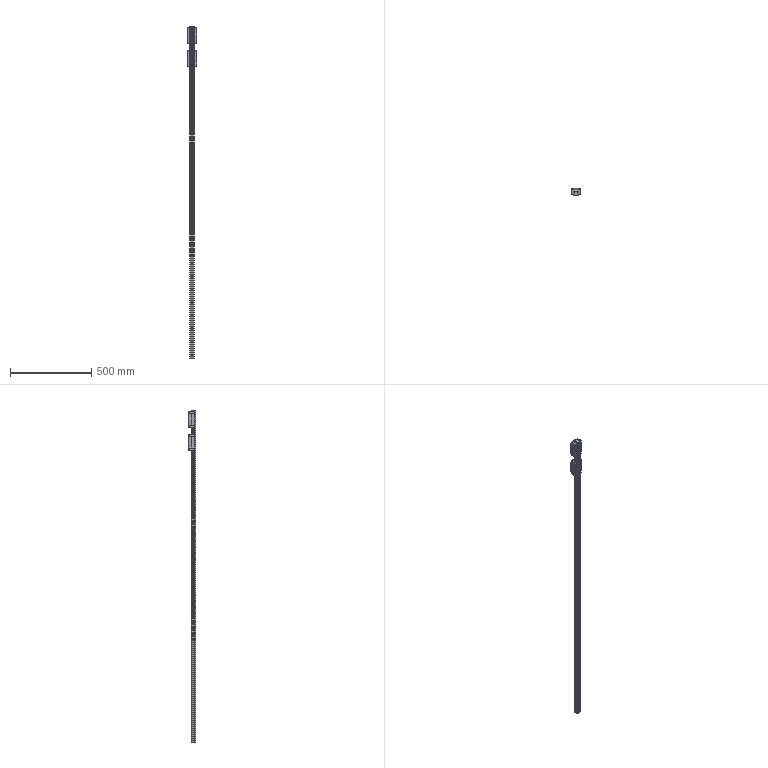Part | SolidWorks | 3 solids | 962 faces | box 60 x 45 x 2040 mm | volume 1527513 mm3 | plane 660 | cylinder 182 | spline 120 | commonest cylinder face diameters 9 x52 14 x52 1.2 x36 8 x16 1.6 x14 5.66 x12